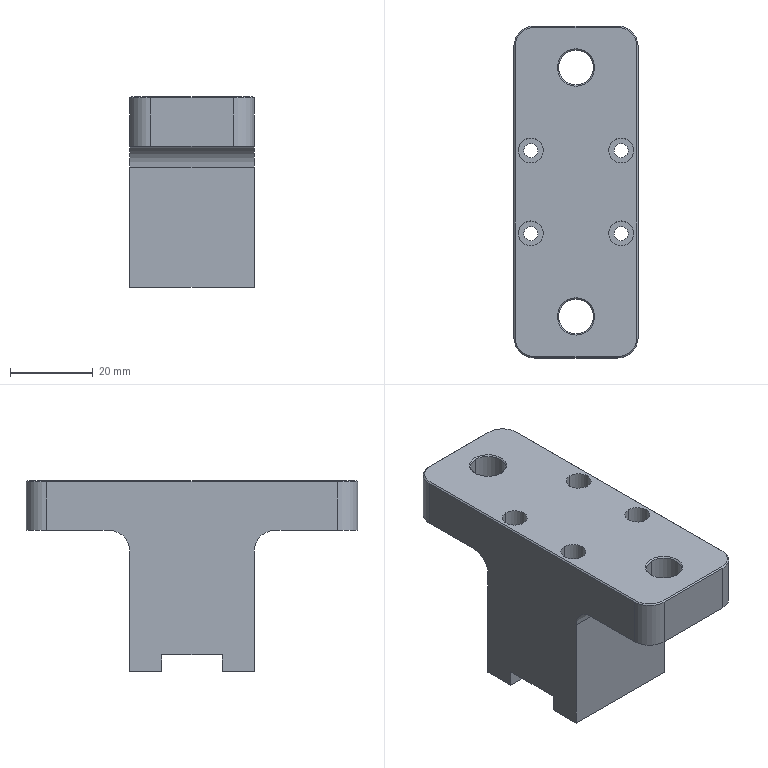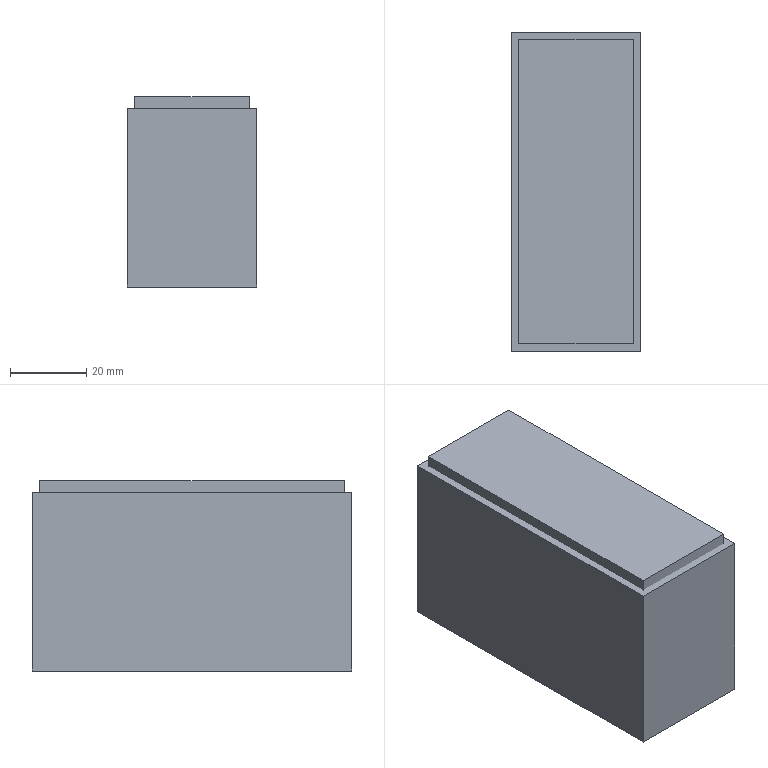CAM job | NX | 3-axis milling, drilling | part box 30 x 80 x 46 mm | stock box 34 x 84 x 50 mm
Tools:
number,name,description,diameter,corner_radius,flute_length,length,flutes
19,D80,Milling Tool-5 Parameters,80.0,0.0,50.0,75.0,2
15,D10,Milling Tool-5 Parameters,10.0,0.0,50.0,75.0,2
14,D10JING,Milling Tool-5 Parameters,10.0,0.0,50.0,75.0,2
16,D6R0.5,Milling Tool-5 Parameters,6.0,0.5,50.0,75.0,2
1,D6A45,Milling Tool-5 Parameters,6.0,0.0,50.0,75.0,2
3,3.4ZT,Drilling Tool,3.4,0.0,35.0,50.0,2
20,8.4ZT,Drilling Tool,8.4,0.0,35.0,50.0,2
6,6.0ZT,Drilling Tool,6.0,0.0,35.0,50.0,2
Operations:
program,operation,operation_type,tool,method,geometry_group,spindle_rpm,surface_speed,feed_per_tooth,feed_cut,feed_plunge,cut_length_mm,path_length_mm,cut_time_min,machine_time_min
1,FLOOR_WALL_COPY,VolumeBased25DMillingOperation,D80,METHOD,A,6500.0,1633.0,0.1154,1500.0,100.0,180.0,234.0,0.12,0.1254
1,ZLEVEL_PROFILE,ZLevelMilling,D10,METHOD,A,9500.0,298.0,0.1579,3000.0,1000.0,11306.119,11409.119,3.801,3.811
1,ZLEVEL_PROFILE_COPY_COPY_COPY,ZLevelMilling,D10,METHOD,A,9500.0,298.0,0.1579,3000.0,1000.0,3105.79,3462.383,1.16,1.196
1,ZLEVEL_PROFILE_COPY_COPY,ZLevelMilling,D10,METHOD,A,9500.0,298.0,0.1579,3000.0,1000.0,3136.677,3477.866,1.169,1.203
1,ZLEVEL_PROFILE_COPY,ZLevelMilling,D10,METHOD,A,9500.0,298.0,0.1579,3000.0,1000.0,3123.446,3449.941,1.16,1.192
1,ZLEVEL_PROFILE_COPY_COPY_1,ZLevelMilling,D10,METHOD,A,9500.0,298.0,0.1579,3000.0,1000.0,371.888,440.358,0.1378,0.1447
1,ZLEVEL_PROFILE_COPY_1_COPY_COPY_1,ZLevelMilling,D10JING,METHOD,A,9500.0,298.0,0.0632,1200.0,1000.0,750.769,901.513,0.6275,0.6425
1,ZLEVEL_PROFILE_COPY_1_COPY_COPY_1_COPY,ZLevelMilling,D10JING,METHOD,A,9500.0,298.0,0.0632,1200.0,1000.0,191.034,529.734,0.1616,0.1955
1,FLOOR_WALL,VolumeBased25DMillingOperation,D10JING,METHOD,A,9500.0,298.0,0.0658,1250.0,100.0,670.783,1397.551,0.5366,0.6093
1,ZLEVEL_PROFILE_1,ZLevelMilling,D6R0.5,METHOD,A,9500.0,119.0,0.1842,3500.0,100.0,4436.347,4715.587,1.268,1.296
1,DRILLING_COPY_1,Operation,D6A45,METHOD,A,5000.0,94.0,0.035,350.0,0.0,28.8,346.752,0.0823,0.1141
1,DRILLING_COPY_1_COPY,Operation,3.4ZT,METHOD,A,2000.0,21.0,0.025,100.0,0.0,208.086,547.625,2.081,2.115
1,DRILLING_COPY_1_COPY_COPY,Operation,8.4ZT,METHOD,A,2000.0,21.0,0.025,100.0,0.0,38.047,267.169,0.3805,0.4034
1,PLANAR_MILL_COPY_COPY_COPY_COPY_COPY_COPY_1_COPY_1,PlanarMilling,D6A45,METHOD,A,9500.0,179.0,0.0658,1250.0,100.0,215.496,641.266,0.1724,0.215
1,PLANAR_MILL_COPY_COPY_COPY_COPY_COPY_COPY_1_COPY_1_COPY,PlanarMilling,D6A45,METHOD,A,9500.0,179.0,0.0658,1250.0,100.0,195.744,786.21,0.1566,0.2156
2,FLOOR_WALL_COPY_COPY,VolumeBased25DMillingOperation,D80,METHOD,B,6500.0,1633.0,0.1154,1500.0,100.0,704.0,1418.001,0.4693,0.5407
2,DRILLING_COPY_1_COPY_COPY_COPY,Operation,6.0ZT,METHOD,B,2000.0,21.0,0.025,100.0,0.0,155.21,449.604,1.552,1.581
2,PLANAR_MILL_COPY_COPY_COPY_COPY_COPY_COPY_1_COPY_1_COPY_1,PlanarMilling,D6A45,METHOD,B,9500.0,179.0,0.0658,1250.0,100.0,353.262,900.599,0.2826,0.3373